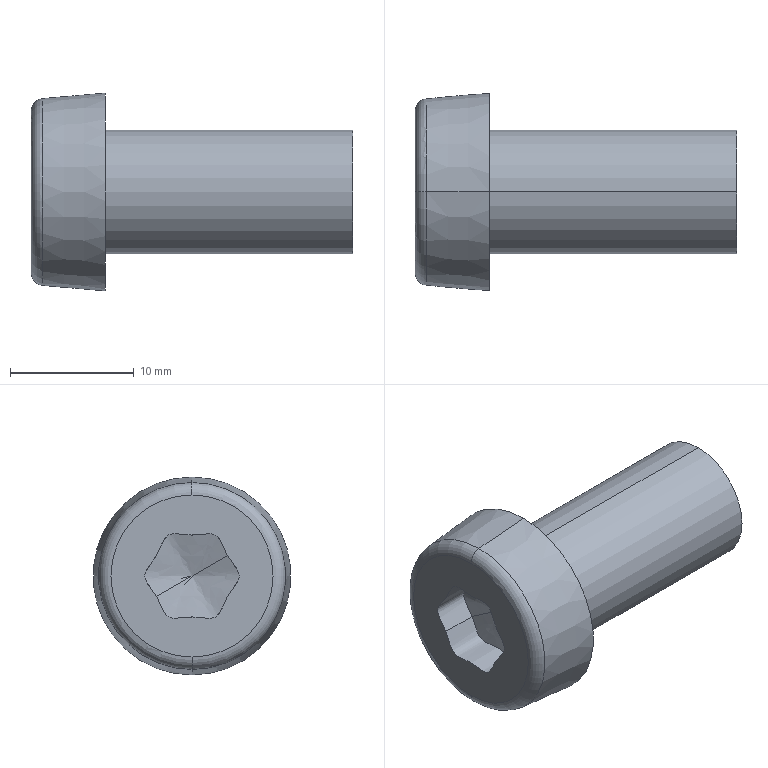Part | SolidWorks | features BlendCut 1, Cut 1, Extrusion 1, Fillet 1, LPattern 1, RevCut 1, Revolution 1 | 1 solid | 13 faces | box 26 x 16 x 16 mm | volume 2561 mm3 | spline 4 | plane 3 | torus 2 | cylinder 2 | cone 2 | commonest cylinder face diameters 10 x2
STEP:
#1=CARTESIAN_POINT('',(0.,0.,6.559));
#2=VERTEX_POINT('',#1);
#3=CARTESIAN_POINT('',(0.,0.,-6.559));
#4=VERTEX_POINT('',#3);
#5=CARTESIAN_POINT('',(0.,0.,0.));
#6=DIRECTION('',(-1.,0.,0.));
#7=DIRECTION('',(0.,0.,-1.));
#8=AXIS2_PLACEMENT_3D('',#5,#6,#7);
#9=CIRCLE('',#8,6.559);
#10=EDGE_CURVE('',#2,#4,#9,.T.);
#11=ORIENTED_EDGE('',*,*,#10,.F.);
#12=CARTESIAN_POINT('',(0.9128,0.,7.555));
#13=VERTEX_POINT('',#12);
#14=CARTESIAN_POINT('',(1.,0.,6.559));
#15=DIRECTION('',(0.,1.,0.));
#16=DIRECTION('',(0.,0.,1.));
#17=AXIS2_PLACEMENT_3D('',#14,#15,#16);
#18=CIRCLE('',#17,1.);
#19=EDGE_CURVE('',#2,#13,#18,.T.);
#20=ORIENTED_EDGE('',*,*,#19,.T.);
#21=CARTESIAN_POINT('',(0.9128,0.,-7.555));
#22=VERTEX_POINT('',#21);
#23=CARTESIAN_POINT('',(0.9128,0.,0.));
#24=DIRECTION('',(1.,0.,0.));
#25=DIRECTION('',(0.,0.,-1.));
#26=AXIS2_PLACEMENT_3D('',#23,#24,#25);
#27=CIRCLE('',#26,7.555);
#28=EDGE_CURVE('',#22,#13,#27,.T.);
#29=ORIENTED_EDGE('',*,*,#28,.F.);
#30=CARTESIAN_POINT('',(1.,0.,-6.559));
#31=DIRECTION('',(0.,-1.,0.));
#32=DIRECTION('',(0.,0.,-1.));
#33=AXIS2_PLACEMENT_3D('',#30,#31,#32);
#34=CIRCLE('',#33,1.);
#35=EDGE_CURVE('',#4,#22,#34,.T.);
#36=ORIENTED_EDGE('',*,*,#35,.F.);
#37=EDGE_LOOP('',(#11,#20,#29,#36));
#38=FACE_OUTER_BOUND('',#37,.T.);
#39=CARTESIAN_POINT('',(1.,0.,0.));
#40=DIRECTION('',(1.,0.,0.));
#41=DIRECTION('',(0.,0.,-1.));
#42=AXIS2_PLACEMENT_3D('',#39,#40,#41);
#43=TOROIDAL_SURFACE('',#42,6.559,1.);
#44=ADVANCED_FACE('',(#38),#43,.T.);
#45=CARTESIAN_POINT('',(4.,0.,0.));
#46=VERTEX_POINT('',#45);
#47=CARTESIAN_POINT('',(3.,2.867,-1.655));
#48=VERTEX_POINT('',#47);
#49=CARTESIAN_POINT('',(4.,0.,0.));
#50=CARTESIAN_POINT('',(3.,2.867,-1.655));
#51=B_SPLINE_CURVE_WITH_KNOTS('',1,(#49,#50),.UNSPECIFIED.,.F.,.F.,(2,2),(0.,1.),.UNSPECIFIED.);
#52=EDGE_CURVE('',#46,#48,#51,.T.);
#53=ORIENTED_EDGE('',*,*,#52,.F.);
#54=CARTESIAN_POINT('',(3.,-2.867,1.655));
#55=VERTEX_POINT('',#54);
#56=CARTESIAN_POINT('',(4.,0.,0.));
#57=CARTESIAN_POINT('',(3.,-2.867,1.655));
#58=B_SPLINE_CURVE_WITH_KNOTS('',1,(#56,#57),.UNSPECIFIED.,.F.,.F.,(2,2),(0.,1.),.UNSPECIFIED.);
#59=EDGE_CURVE('',#46,#55,#58,.T.);
#60=ORIENTED_EDGE('',*,*,#59,.T.);
#61=CARTESIAN_POINT('',(3.,-2.867,1.655));
#62=CARTESIAN_POINT('',(3.,-2.499,2.292));
#63=CARTESIAN_POINT('',(3.,-2.205,3.819));
#64=CARTESIAN_POINT('',(3.,0.,3.055));
#65=CARTESIAN_POINT('',(3.,2.205,3.819));
#66=CARTESIAN_POINT('',(3.,2.646,1.528));
#67=CARTESIAN_POINT('',(3.,4.41,0.));
#68=CARTESIAN_POINT('',(3.,3.234,-1.018));
#69=CARTESIAN_POINT('',(3.,2.867,-1.655));
#70=B_SPLINE_CURVE_WITH_KNOTS('',3,(#61,#62,#63,#64,#65,#66,#67,#68,#69),.UNSPECIFIED.,.F.,.F.,(4,1,1,1,1,1,4),(0.5,0.5833,0.6667,0.75,0.8333,0.9167,1.),.UNSPECIFIED.);
#71=EDGE_CURVE('',#55,#48,#70,.T.);
#72=ORIENTED_EDGE('',*,*,#71,.T.);
#73=EDGE_LOOP('',(#53,#60,#72));
#74=FACE_OUTER_BOUND('',#73,.T.);
#75=CARTESIAN_POINT('',(4.,0.,0.));
#76=CARTESIAN_POINT('',(3.,2.867,-1.655));
#77=CARTESIAN_POINT('',(4.,0.,0.));
#78=CARTESIAN_POINT('',(3.,2.499,-2.292));
#79=CARTESIAN_POINT('',(4.,0.,0.));
#80=CARTESIAN_POINT('',(3.,2.205,-3.819));
#81=CARTESIAN_POINT('',(4.,0.,0.));
#82=CARTESIAN_POINT('',(3.,0.,-3.055));
#83=CARTESIAN_POINT('',(4.,0.,0.));
#84=CARTESIAN_POINT('',(3.,-2.205,-3.819));
#85=CARTESIAN_POINT('',(4.,0.,0.));
#86=CARTESIAN_POINT('',(3.,-2.646,-1.528));
#87=CARTESIAN_POINT('',(4.,0.,0.));
#88=CARTESIAN_POINT('',(3.,-4.41,0.));
#89=CARTESIAN_POINT('',(4.,0.,0.));
#90=CARTESIAN_POINT('',(3.,-2.646,1.528));
#91=CARTESIAN_POINT('',(4.,0.,0.));
#92=CARTESIAN_POINT('',(3.,-2.205,3.819));
#93=CARTESIAN_POINT('',(4.,0.,0.));
#94=CARTESIAN_POINT('',(3.,0.,3.055));
#95=CARTESIAN_POINT('',(4.,0.,0.));
#96=CARTESIAN_POINT('',(3.,2.205,3.819));
#97=CARTESIAN_POINT('',(4.,0.,0.));
#98=CARTESIAN_POINT('',(3.,2.646,1.528));
#99=CARTESIAN_POINT('',(4.,0.,0.));
#100=CARTESIAN_POINT('',(3.,4.41,0.));
#101=CARTESIAN_POINT('',(4.,0.,0.));
#102=CARTESIAN_POINT('',(3.,3.234,-1.018));
#103=CARTESIAN_POINT('',(4.,0.,0.));
#104=CARTESIAN_POINT('',(3.,2.867,-1.655));
#105=B_SPLINE_SURFACE_WITH_KNOTS('',3,1,((#75,#76),(#77,#78),(#79,#80),(#81,#82),(#83,#84),(#85,#86),(#87,#88),(#89,#90),(#91,#92),(#93,#94),(#95,#96),(#97,#98),(#99,#100),(#101,#102),(#103,#104)),.UNSPECIFIED.,.T.,.F.,.F.,(4,1,1,1,1,1,1,1,1,1,1,1,4),(2,2),(0.,0.08333,0.1667,0.25,0.3333,0.4167,0.5,0.5833,0.6667,0.75,0.8333,0.9167,1.),(0.,1.),.UNSPECIFIED.);
#106=ADVANCED_FACE('',(#74),#105,.F.);
#107=ORIENTED_EDGE('',*,*,#71,.F.);
#108=CARTESIAN_POINT('',(0.,-2.867,1.655));
#109=VERTEX_POINT('',#108);
#110=CARTESIAN_POINT('',(3.,-2.867,1.655));
#111=DIRECTION('',(-1.,0.,0.));
#112=VECTOR('',#111,1000.);
#113=LINE('',#110,#112);
#114=EDGE_CURVE('',#55,#109,#113,.T.);
#115=ORIENTED_EDGE('',*,*,#114,.T.);
#116=CARTESIAN_POINT('',(0.,2.867,-1.655));
#117=VERTEX_POINT('',#116);
#118=CARTESIAN_POINT('',(0.,2.867,-1.655));
#119=CARTESIAN_POINT('',(0.,3.234,-1.018));
#120=CARTESIAN_POINT('',(0.,4.41,0.));
#121=CARTESIAN_POINT('',(0.,2.646,1.528));
#122=CARTESIAN_POINT('',(0.,2.205,3.819));
#123=CARTESIAN_POINT('',(0.,0.,3.055));
#124=CARTESIAN_POINT('',(0.,-2.205,3.819));
#125=CARTESIAN_POINT('',(0.,-2.499,2.292));
#126=CARTESIAN_POINT('',(0.,-2.867,1.655));
#127=B_SPLINE_CURVE_WITH_KNOTS('',3,(#118,#119,#120,#121,#122,#123,#124,#125,#126),.UNSPECIFIED.,.F.,.F.,(4,1,1,1,1,1,4),(0.,0.08333,0.1667,0.25,0.3333,0.4167,0.5),.UNSPECIFIED.);
#128=EDGE_CURVE('',#117,#109,#127,.T.);
#129=ORIENTED_EDGE('',*,*,#128,.F.);
#130=CARTESIAN_POINT('',(3.,2.867,-1.655));
#131=DIRECTION('',(-1.,0.,0.));
#132=VECTOR('',#131,1000.);
#133=LINE('',#130,#132);
#134=EDGE_CURVE('',#48,#117,#133,.T.);
#135=ORIENTED_EDGE('',*,*,#134,.F.);
#136=EDGE_LOOP('',(#107,#115,#129,#135));
#137=FACE_OUTER_BOUND('',#136,.T.);
#138=CARTESIAN_POINT('',(3.,2.867,-1.655));
#139=CARTESIAN_POINT('',(0.,2.867,-1.655));
#140=CARTESIAN_POINT('',(3.,3.234,-1.018));
#141=CARTESIAN_POINT('',(0.,3.234,-1.018));
#142=CARTESIAN_POINT('',(3.,4.41,0.));
#143=CARTESIAN_POINT('',(0.,4.41,0.));
#144=CARTESIAN_POINT('',(3.,2.646,1.528));
#145=CARTESIAN_POINT('',(0.,2.646,1.528));
#146=CARTESIAN_POINT('',(3.,2.205,3.819));
#147=CARTESIAN_POINT('',(0.,2.205,3.819));
#148=CARTESIAN_POINT('',(3.,0.,3.055));
#149=CARTESIAN_POINT('',(0.,0.,3.055));
#150=CARTESIAN_POINT('',(3.,-2.205,3.819));
#151=CARTESIAN_POINT('',(0.,-2.205,3.819));
#152=CARTESIAN_POINT('',(3.,-2.499,2.292));
#153=CARTESIAN_POINT('',(0.,-2.499,2.292));
#154=CARTESIAN_POINT('',(3.,-2.867,1.655));
#155=CARTESIAN_POINT('',(0.,-2.867,1.655));
#156=B_SPLINE_SURFACE_WITH_KNOTS('',3,1,((#138,#139),(#140,#141),(#142,#143),(#144,#145),(#146,#147),(#148,#149),(#150,#151),(#152,#153),(#154,#155)),.UNSPECIFIED.,.F.,.F.,.F.,(4,1,1,1,1,1,4),(2,2),(0.,0.08333,0.1667,0.25,0.3333,0.4167,0.5),(0.,1.),.UNSPECIFIED.);
#157=ADVANCED_FACE('',(#137),#156,.T.);
#158=CARTESIAN_POINT('',(26.,0.,5.));
#159=VERTEX_POINT('',#158);
#160=CARTESIAN_POINT('',(26.,0.,-5.));
#161=VERTEX_POINT('',#160);
#162=CARTESIAN_POINT('',(26.,0.,0.));
#163=DIRECTION('',(-1.,0.,0.));
#164=DIRECTION('',(0.,0.,1.));
#165=AXIS2_PLACEMENT_3D('',#162,#163,#164);
#166=CIRCLE('',#165,5.);
#167=EDGE_CURVE('',#159,#161,#166,.T.);
#168=ORIENTED_EDGE('',*,*,#167,.T.);
#169=CARTESIAN_POINT('',(6.,0.,-5.));
#170=VERTEX_POINT('',#169);
#171=CARTESIAN_POINT('',(0.,0.,-5.));
#172=DIRECTION('',(-1.,0.,0.));
#173=VECTOR('',#172,1000.);
#174=LINE('',#171,#173);
#175=EDGE_CURVE('',#161,#170,#174,.T.);
#176=ORIENTED_EDGE('',*,*,#175,.T.);
#177=CARTESIAN_POINT('',(6.,0.,5.));
#178=VERTEX_POINT('',#177);
#179=CARTESIAN_POINT('',(6.,0.,0.));
#180=DIRECTION('',(-1.,0.,0.));
#181=DIRECTION('',(0.,0.,1.));
#182=AXIS2_PLACEMENT_3D('',#179,#180,#181);
#183=CIRCLE('',#182,5.);
#184=EDGE_CURVE('',#178,#170,#183,.T.);
#185=ORIENTED_EDGE('',*,*,#184,.F.);
#186=CARTESIAN_POINT('',(0.,0.,5.));
#187=DIRECTION('',(-1.,0.,0.));
#188=VECTOR('',#187,1000.);
#189=LINE('',#186,#188);
#190=EDGE_CURVE('',#159,#178,#189,.T.);
#191=ORIENTED_EDGE('',*,*,#190,.F.);
#192=EDGE_LOOP('',(#168,#176,#185,#191));
#193=FACE_OUTER_BOUND('',#192,.T.);
#194=CARTESIAN_POINT('',(0.,0.,0.));
#195=DIRECTION('',(-1.,0.,0.));
#196=DIRECTION('',(0.,0.,1.));
#197=AXIS2_PLACEMENT_3D('',#194,#195,#196);
#198=CYLINDRICAL_SURFACE('',#197,5.);
#199=ADVANCED_FACE('',(#193),#198,.T.);
#200=ORIENTED_EDGE('',*,*,#28,.T.);
#201=CARTESIAN_POINT('',(6.,0.,8.));
#202=VERTEX_POINT('',#201);
#203=CARTESIAN_POINT('',(6.,0.,8.));
#204=DIRECTION('',(0.9962,0.,0.08716));
#205=VECTOR('',#204,1000.);
#206=LINE('',#203,#205);
#207=EDGE_CURVE('',#13,#202,#206,.T.);
#208=ORIENTED_EDGE('',*,*,#207,.T.);
#209=CARTESIAN_POINT('',(6.,0.,-8.));
#210=VERTEX_POINT('',#209);
#211=CARTESIAN_POINT('',(6.,0.,0.));
#212=DIRECTION('',(1.,0.,0.));
#213=DIRECTION('',(0.,0.,-1.));
#214=AXIS2_PLACEMENT_3D('',#211,#212,#213);
#215=CIRCLE('',#214,8.);
#216=EDGE_CURVE('',#210,#202,#215,.T.);
#217=ORIENTED_EDGE('',*,*,#216,.F.);
#218=CARTESIAN_POINT('',(6.,0.,-8.));
#219=DIRECTION('',(0.9962,0.,-0.08716));
#220=VECTOR('',#219,1000.);
#221=LINE('',#218,#220);
#222=EDGE_CURVE('',#22,#210,#221,.T.);
#223=ORIENTED_EDGE('',*,*,#222,.F.);
#224=EDGE_LOOP('',(#200,#208,#217,#223));
#225=FACE_OUTER_BOUND('',#224,.T.);
#226=CARTESIAN_POINT('',(6.,0.,0.));
#227=DIRECTION('',(1.,0.,0.));
#228=DIRECTION('',(0.,0.,-1.));
#229=AXIS2_PLACEMENT_3D('',#226,#227,#228);
#230=CONICAL_SURFACE('',#229,8.,0.08727);
#231=ADVANCED_FACE('',(#225),#230,.T.);
#232=CARTESIAN_POINT('',(0.,0.,0.));
#233=DIRECTION('',(-1.,0.,0.));
#234=DIRECTION('',(0.,0.,-1.));
#235=AXIS2_PLACEMENT_3D('',#232,#233,#234);
#236=CIRCLE('',#235,6.559);
#237=EDGE_CURVE('',#4,#2,#236,.T.);
#238=ORIENTED_EDGE('',*,*,#237,.T.);
#239=ORIENTED_EDGE('',*,*,#10,.T.);
#240=EDGE_LOOP('',(#238,#239));
#241=FACE_OUTER_BOUND('',#240,.T.);
#242=ORIENTED_EDGE('',*,*,#128,.T.);
#243=CARTESIAN_POINT('',(0.,-2.867,1.655));
#244=CARTESIAN_POINT('',(0.,-3.234,1.018));
#245=CARTESIAN_POINT('',(0.,-4.41,0.));
#246=CARTESIAN_POINT('',(0.,-2.646,-1.528));
#247=CARTESIAN_POINT('',(0.,-2.205,-3.819));
#248=CARTESIAN_POINT('',(0.,0.,-3.055));
#249=CARTESIAN_POINT('',(0.,2.205,-3.819));
#250=CARTESIAN_POINT('',(0.,2.499,-2.292));
#251=CARTESIAN_POINT('',(0.,2.867,-1.655));
#252=B_SPLINE_CURVE_WITH_KNOTS('',3,(#243,#244,#245,#246,#247,#248,#249,#250,#251),.UNSPECIFIED.,.F.,.F.,(4,1,1,1,1,1,4),(0.5,0.5833,0.6667,0.75,0.8333,0.9167,1.),.UNSPECIFIED.);
#253=EDGE_CURVE('',#109,#117,#252,.T.);
#254=ORIENTED_EDGE('',*,*,#253,.T.);
#255=EDGE_LOOP('',(#242,#254));
#256=FACE_BOUND('',#255,.T.);
#257=CARTESIAN_POINT('',(0.,0.,0.));
#258=DIRECTION('',(1.,0.,0.));
#259=DIRECTION('',(0.,0.,-1.));
#260=AXIS2_PLACEMENT_3D('',#257,#258,#259);
#261=PLANE('',#260);
#262=ADVANCED_FACE('',(#241,#256),#261,.F.);
#263=ORIENTED_EDGE('',*,*,#216,.T.);
#264=CARTESIAN_POINT('',(6.,0.,0.));
#265=DIRECTION('',(1.,0.,0.));
#266=DIRECTION('',(0.,0.,-1.));
#267=AXIS2_PLACEMENT_3D('',#264,#265,#266);
#268=CIRCLE('',#267,8.);
#269=EDGE_CURVE('',#202,#210,#268,.T.);
#270=ORIENTED_EDGE('',*,*,#269,.T.);
#271=EDGE_LOOP('',(#263,#270));
#272=FACE_OUTER_BOUND('',#271,.T.);
#273=ORIENTED_EDGE('',*,*,#184,.T.);
#274=CARTESIAN_POINT('',(6.,0.,0.));
#275=DIRECTION('',(-1.,0.,0.));
#276=DIRECTION('',(0.,0.,1.));
#277=AXIS2_PLACEMENT_3D('',#274,#275,#276);
#278=CIRCLE('',#277,5.);
#279=EDGE_CURVE('',#170,#178,#278,.T.);
#280=ORIENTED_EDGE('',*,*,#279,.T.);
#281=EDGE_LOOP('',(#273,#280));
#282=FACE_BOUND('',#281,.T.);
#283=CARTESIAN_POINT('',(6.,0.,0.));
#284=DIRECTION('',(1.,0.,0.));
#285=DIRECTION('',(0.,0.,-1.));
#286=AXIS2_PLACEMENT_3D('',#283,#284,#285);
#287=PLANE('',#286);
#288=ADVANCED_FACE('',(#272,#282),#287,.T.);
#289=ORIENTED_EDGE('',*,*,#207,.F.);
#290=CARTESIAN_POINT('',(0.9128,0.,0.));
#291=DIRECTION('',(1.,0.,0.));
#292=DIRECTION('',(0.,0.,-1.));
#293=AXIS2_PLACEMENT_3D('',#290,#291,#292);
#294=CIRCLE('',#293,7.555);
#295=EDGE_CURVE('',#13,#22,#294,.T.);
#296=ORIENTED_EDGE('',*,*,#295,.T.);
#297=ORIENTED_EDGE('',*,*,#222,.T.);
#298=ORIENTED_EDGE('',*,*,#269,.F.);
#299=EDGE_LOOP('',(#289,#296,#297,#298));
#300=FACE_OUTER_BOUND('',#299,.T.);
#301=CARTESIAN_POINT('',(6.,0.,0.));
#302=DIRECTION('',(1.,0.,0.));
#303=DIRECTION('',(0.,0.,-1.));
#304=AXIS2_PLACEMENT_3D('',#301,#302,#303);
#305=CONICAL_SURFACE('',#304,8.,0.08727);
#306=ADVANCED_FACE('',(#300),#305,.T.);
#307=ORIENTED_EDGE('',*,*,#167,.F.);
#308=CARTESIAN_POINT('',(26.,0.,0.));
#309=DIRECTION('',(-1.,0.,0.));
#310=DIRECTION('',(0.,0.,1.));
#311=AXIS2_PLACEMENT_3D('',#308,#309,#310);
#312=CIRCLE('',#311,5.);
#313=EDGE_CURVE('',#161,#159,#312,.T.);
#314=ORIENTED_EDGE('',*,*,#313,.F.);
#315=EDGE_LOOP('',(#307,#314));
#316=FACE_OUTER_BOUND('',#315,.T.);
#317=CARTESIAN_POINT('',(26.,5.,0.));
#318=DIRECTION('',(-1.,0.,0.));
#319=DIRECTION('',(0.,0.,1.));
#320=AXIS2_PLACEMENT_3D('',#317,#318,#319);
#321=PLANE('',#320);
#322=ADVANCED_FACE('',(#316),#321,.F.);
#323=ORIENTED_EDGE('',*,*,#175,.F.);
#324=ORIENTED_EDGE('',*,*,#313,.T.);
#325=ORIENTED_EDGE('',*,*,#190,.T.);
#326=ORIENTED_EDGE('',*,*,#279,.F.);
#327=EDGE_LOOP('',(#323,#324,#325,#326));
#328=FACE_OUTER_BOUND('',#327,.T.);
#329=CARTESIAN_POINT('',(0.,0.,0.));
#330=DIRECTION('',(-1.,0.,0.));
#331=DIRECTION('',(0.,0.,1.));
#332=AXIS2_PLACEMENT_3D('',#329,#330,#331);
#333=CYLINDRICAL_SURFACE('',#332,5.);
#334=ADVANCED_FACE('',(#328),#333,.T.);
#335=ORIENTED_EDGE('',*,*,#114,.F.);
#336=CARTESIAN_POINT('',(3.,2.867,-1.655));
#337=CARTESIAN_POINT('',(3.,2.499,-2.292));
#338=CARTESIAN_POINT('',(3.,2.205,-3.819));
#339=CARTESIAN_POINT('',(3.,0.,-3.055));
#340=CARTESIAN_POINT('',(3.,-2.205,-3.819));
#341=CARTESIAN_POINT('',(3.,-2.646,-1.528));
#342=CARTESIAN_POINT('',(3.,-4.41,0.));
#343=CARTESIAN_POINT('',(3.,-3.234,1.018));
#344=CARTESIAN_POINT('',(3.,-2.867,1.655));
#345=B_SPLINE_CURVE_WITH_KNOTS('',3,(#336,#337,#338,#339,#340,#341,#342,#343,#344),.UNSPECIFIED.,.F.,.F.,(4,1,1,1,1,1,4),(0.,0.08333,0.1667,0.25,0.3333,0.4167,0.5),.UNSPECIFIED.);
#346=EDGE_CURVE('',#48,#55,#345,.T.);
#347=ORIENTED_EDGE('',*,*,#346,.F.);
#348=ORIENTED_EDGE('',*,*,#134,.T.);
#349=ORIENTED_EDGE('',*,*,#253,.F.);
#350=EDGE_LOOP('',(#335,#347,#348,#349));
#351=FACE_OUTER_BOUND('',#350,.T.);
#352=CARTESIAN_POINT('',(3.,-2.867,1.655));
#353=CARTESIAN_POINT('',(0.,-2.867,1.655));
#354=CARTESIAN_POINT('',(3.,-3.234,1.018));
#355=CARTESIAN_POINT('',(0.,-3.234,1.018));
#356=CARTESIAN_POINT('',(3.,-4.41,0.));
#357=CARTESIAN_POINT('',(0.,-4.41,0.));
#358=CARTESIAN_POINT('',(3.,-2.646,-1.528));
#359=CARTESIAN_POINT('',(0.,-2.646,-1.528));
#360=CARTESIAN_POINT('',(3.,-2.205,-3.819));
#361=CARTESIAN_POINT('',(0.,-2.205,-3.819));
#362=CARTESIAN_POINT('',(3.,0.,-3.055));
#363=CARTESIAN_POINT('',(0.,0.,-3.055));
#364=CARTESIAN_POINT('',(3.,2.205,-3.819));
#365=CARTESIAN_POINT('',(0.,2.205,-3.819));
#366=CARTESIAN_POINT('',(3.,2.499,-2.292));
#367=CARTESIAN_POINT('',(0.,2.499,-2.292));
#368=CARTESIAN_POINT('',(3.,2.867,-1.655));
#369=CARTESIAN_POINT('',(0.,2.867,-1.655));
#370=B_SPLINE_SURFACE_WITH_KNOTS('',3,1,((#352,#353),(#354,#355),(#356,#357),(#358,#359),(#360,#361),(#362,#363),(#364,#365),(#366,#367),(#368,#369)),.UNSPECIFIED.,.F.,.F.,.F.,(4,1,1,1,1,1,4),(2,2),(0.5,0.5833,0.6667,0.75,0.8333,0.9167,1.),(0.,1.),.UNSPECIFIED.);
#371=ADVANCED_FACE('',(#351),#370,.T.);
#372=ORIENTED_EDGE('',*,*,#59,.F.);
#373=ORIENTED_EDGE('',*,*,#52,.T.);
#374=ORIENTED_EDGE('',*,*,#346,.T.);
#375=EDGE_LOOP('',(#372,#373,#374));
#376=FACE_OUTER_BOUND('',#375,.T.);
#377=CARTESIAN_POINT('',(4.,0.,0.));
#378=CARTESIAN_POINT('',(3.,2.867,-1.655));
#379=CARTESIAN_POINT('',(4.,0.,0.));
#380=CARTESIAN_POINT('',(3.,2.499,-2.292));
#381=CARTESIAN_POINT('',(4.,0.,0.));
#382=CARTESIAN_POINT('',(3.,2.205,-3.819));
#383=CARTESIAN_POINT('',(4.,0.,0.));
#384=CARTESIAN_POINT('',(3.,0.,-3.055));
#385=CARTESIAN_POINT('',(4.,0.,0.));
#386=CARTESIAN_POINT('',(3.,-2.205,-3.819));
#387=CARTESIAN_POINT('',(4.,0.,0.));
#388=CARTESIAN_POINT('',(3.,-2.646,-1.528));
#389=CARTESIAN_POINT('',(4.,0.,0.));
#390=CARTESIAN_POINT('',(3.,-4.41,0.));
#391=CARTESIAN_POINT('',(4.,0.,0.));
#392=CARTESIAN_POINT('',(3.,-2.646,1.528));
#393=CARTESIAN_POINT('',(4.,0.,0.));
#394=CARTESIAN_POINT('',(3.,-2.205,3.819));
#395=CARTESIAN_POINT('',(4.,0.,0.));
#396=CARTESIAN_POINT('',(3.,0.,3.055));
#397=CARTESIAN_POINT('',(4.,0.,0.));
#398=CARTESIAN_POINT('',(3.,2.205,3.819));
#399=CARTESIAN_POINT('',(4.,0.,0.));
#400=CARTESIAN_POINT('',(3.,2.646,1.528));
#401=CARTESIAN_POINT('',(4.,0.,0.));
#402=CARTESIAN_POINT('',(3.,4.41,0.));
#403=CARTESIAN_POINT('',(4.,0.,0.));
#404=CARTESIAN_POINT('',(3.,3.234,-1.018));
#405=CARTESIAN_POINT('',(4.,0.,0.));
#406=CARTESIAN_POINT('',(3.,2.867,-1.655));
#407=B_SPLINE_SURFACE_WITH_KNOTS('',3,1,((#377,#378),(#379,#380),(#381,#382),(#383,#384),(#385,#386),(#387,#388),(#389,#390),(#391,#392),(#393,#394),(#395,#396),(#397,#398),(#399,#400),(#401,#402),(#403,#404),(#405,#406)),.UNSPECIFIED.,.T.,.F.,.F.,(4,1,1,1,1,1,1,1,1,1,1,1,4),(2,2),(0.,0.08333,0.1667,0.25,0.3333,0.4167,0.5,0.5833,0.6667,0.75,0.8333,0.9167,1.),(0.,1.),.UNSPECIFIED.);
#408=ADVANCED_FACE('',(#376),#407,.F.);
#409=ORIENTED_EDGE('',*,*,#19,.F.);
#410=ORIENTED_EDGE('',*,*,#237,.F.);
#411=ORIENTED_EDGE('',*,*,#35,.T.);
#412=ORIENTED_EDGE('',*,*,#295,.F.);
#413=EDGE_LOOP('',(#409,#410,#411,#412));
#414=FACE_OUTER_BOUND('',#413,.T.);
#415=CARTESIAN_POINT('',(1.,0.,0.));
#416=DIRECTION('',(1.,0.,0.));
#417=DIRECTION('',(0.,0.,-1.));
#418=AXIS2_PLACEMENT_3D('',#415,#416,#417);
#419=TOROIDAL_SURFACE('',#418,6.559,1.);
#420=ADVANCED_FACE('',(#414),#419,.T.);
#421=CLOSED_SHELL('',(#44,#106,#157,#199,#231,#262,#288,#306,#322,#334,#371,#408,#420));
#422=MANIFOLD_SOLID_BREP('',#421);
#423=CARTESIAN_POINT('',(0.,0.,0.));
#424=DIRECTION('',(0.,0.,1.));
#425=DIRECTION('',(1.,0.,0.));
#426=AXIS2_PLACEMENT_3D('',#423,#424,#425);
#427=(LENGTH_UNIT()NAMED_UNIT(*)SI_UNIT(.MILLI.,.METRE.));
#428=UNCERTAINTY_MEASURE_WITH_UNIT(LENGTH_MEASURE(0.00001),#427,'','');
#429=(NAMED_UNIT(*)PLANE_ANGLE_UNIT()SI_UNIT($,.RADIAN.));
#430=(NAMED_UNIT(*)SI_UNIT($,.STERADIAN.)SOLID_ANGLE_UNIT());
#431=(GEOMETRIC_REPRESENTATION_CONTEXT(3)GLOBAL_UNCERTAINTY_ASSIGNED_CONTEXT((#428))GLOBAL_UNIT_ASSIGNED_CONTEXT((#427,#429,#430))REPRESENTATION_CONTEXT('',''));
#432=ADVANCED_BREP_SHAPE_REPRESENTATION('',(#422,#426),#431);